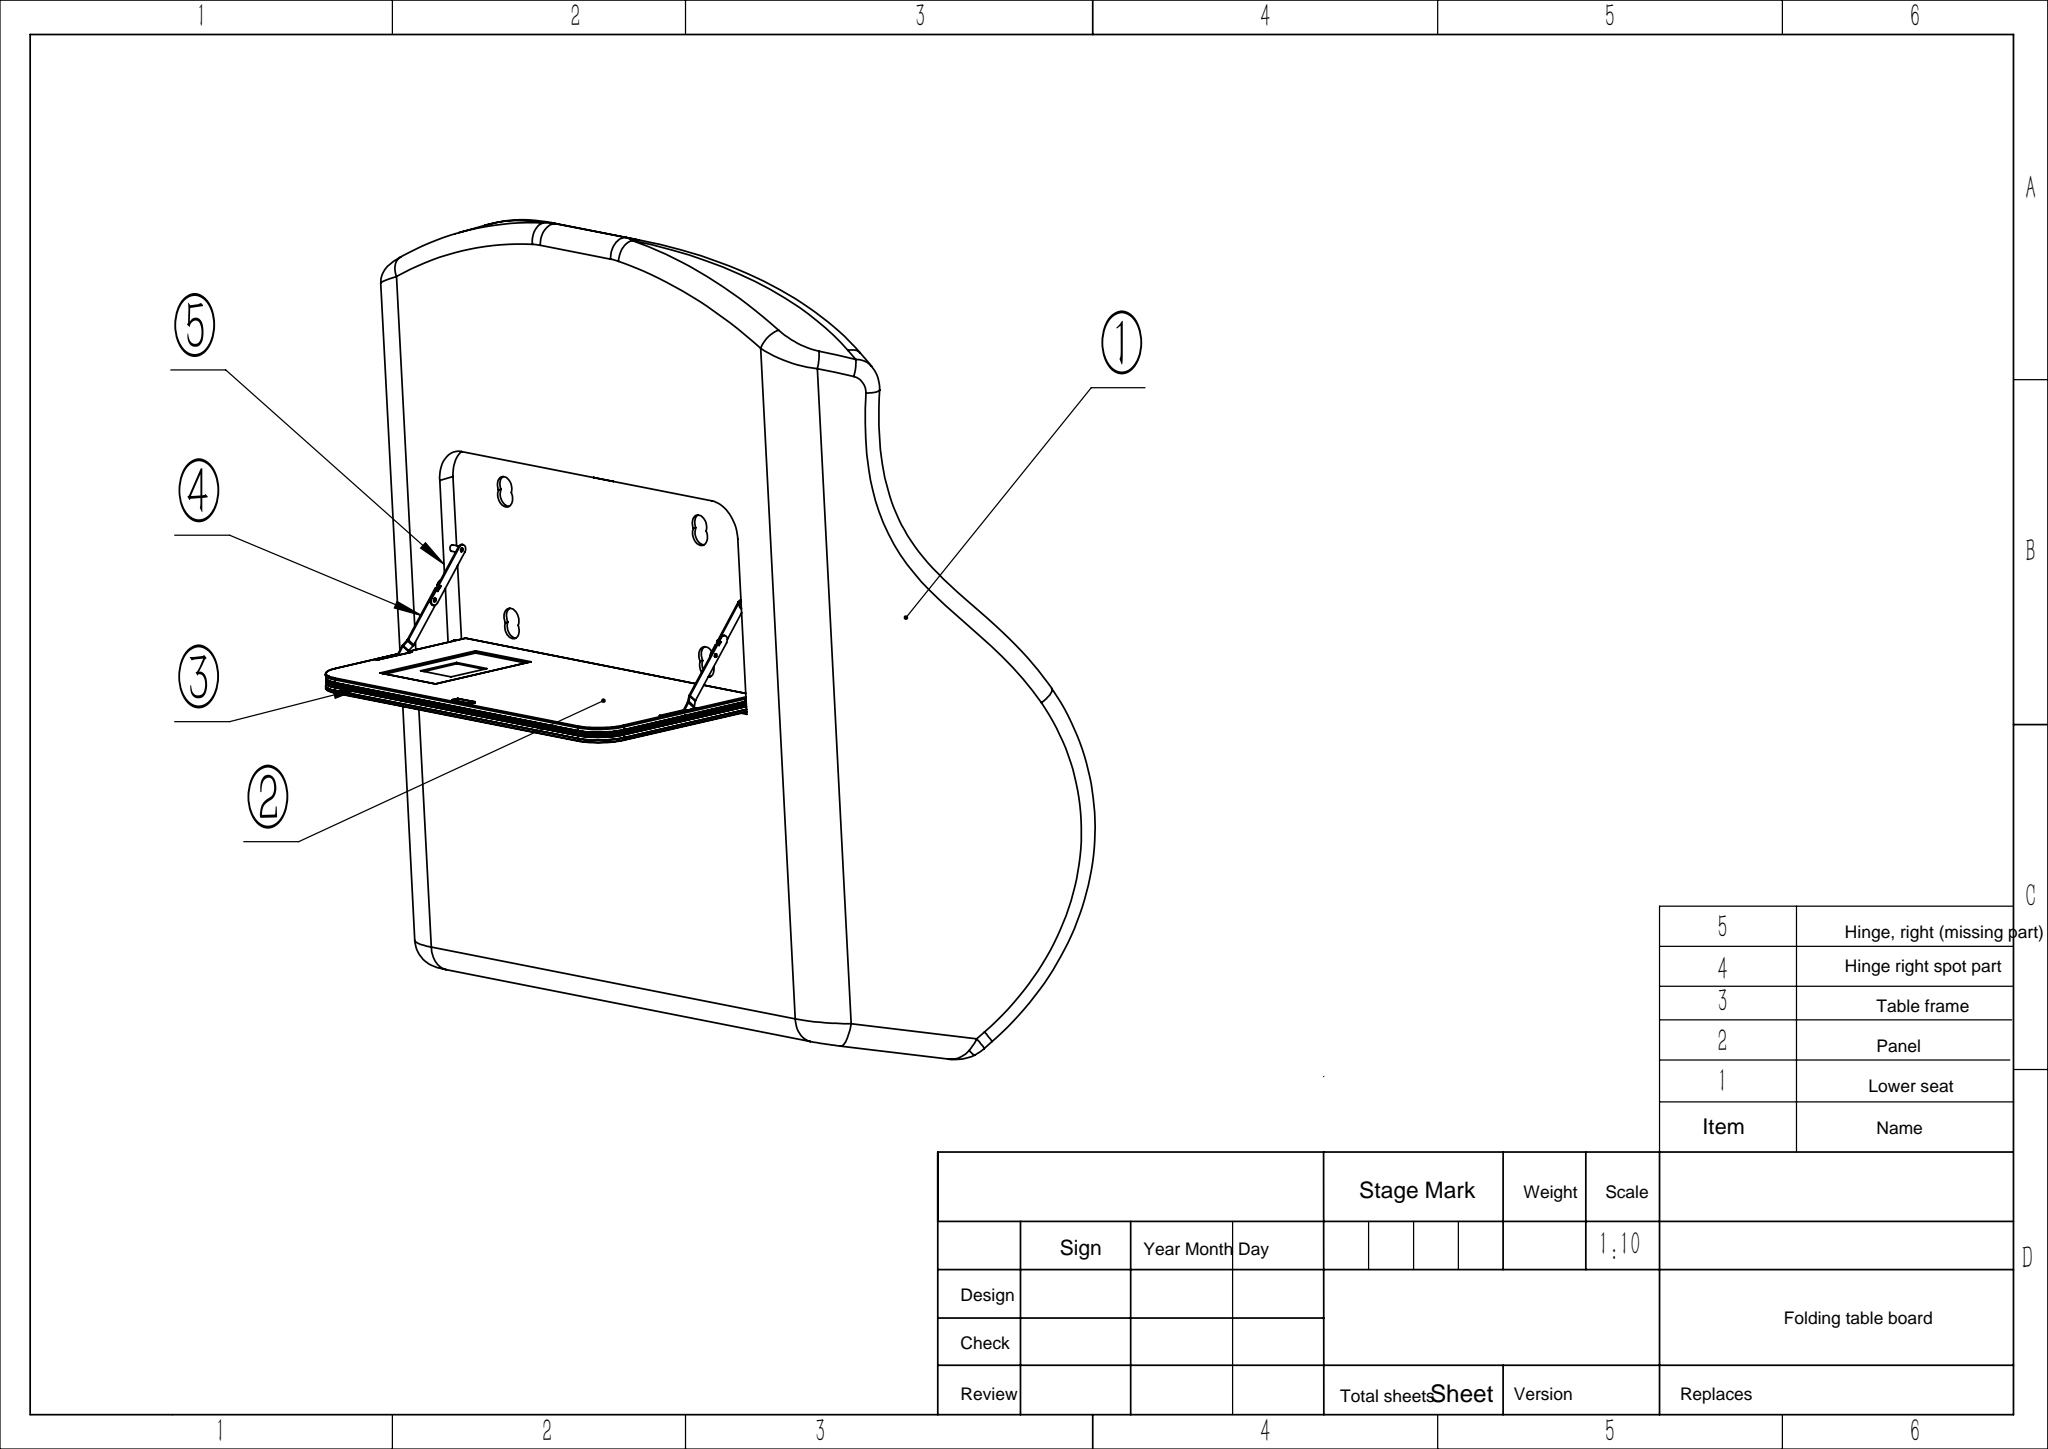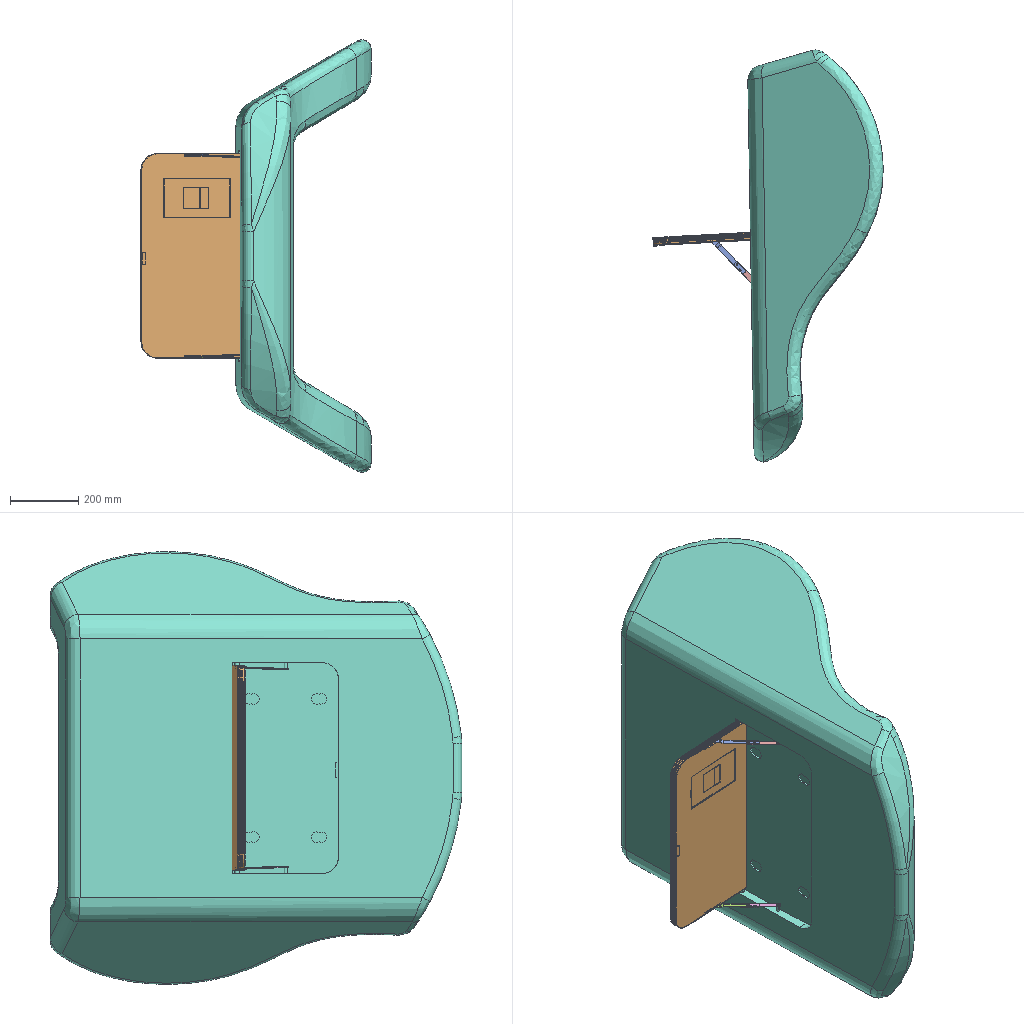Assembly | SolidWorks | 12 different items | 12 placed | box 674 x 1206 x 1267 mm
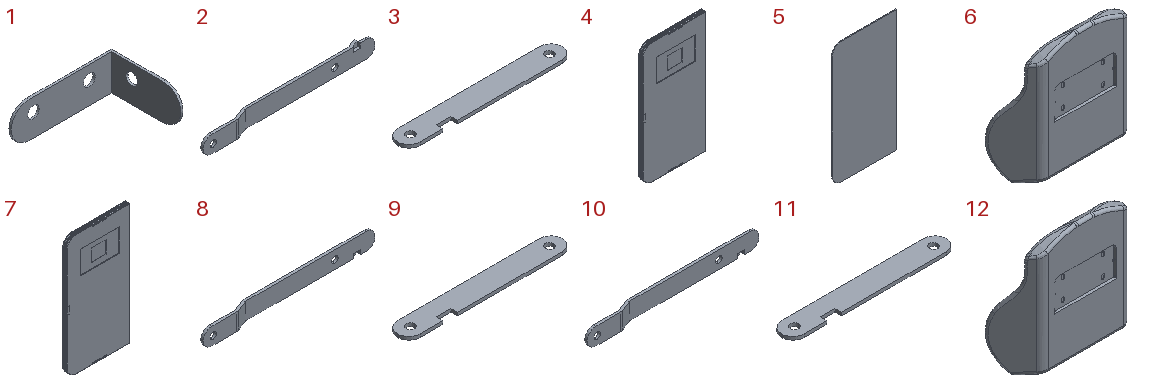Parts list (item | quantity | size | volume | features):
1 | x1 | 46 x 32 x 16 mm | 1113 mm3 | features MirrorStock 1
2 | x1 | 145 x 8.5 x 14 mm | 3916 mm3 | features MirrorStock 1
3 | x1 | 102 x 14 x 2 mm | 2615 mm3 | features MirrorStock 1
4 | x1 | 312 x 24.5 x 600 mm | 4043732 mm3 | features ICE 11, Fillet 4, MirrorPattern 1, Sweep 1
5 | x1 | 315.5 x 4 x 596 mm | 748519 mm3 | features Extrusion 1
6 | x1 | 1267 x 391.764 x 1203 mm | 196548846 mm3 | features ICE 13, MirrorPattern 6, Fillet 5, Extrusion 1, RefAxis 1, Scale 1
7 | x1 | 312 x 24.5 x 600 mm | 4043732 mm3 | features ICE 11, Fillet 4, MirrorPattern 1, Sweep 1
8 | x1 | 145 x 8.5 x 14 mm | 3916 mm3 | features ICE 3, Extrusion 1
9 | x1 | 102 x 14 x 2 mm | 2615 mm3 | features Extrusion 1
10 | x1 | 145 x 8.5 x 14 mm | 3916 mm3 | features ICE 3, Extrusion 1
11 | x1 | 102 x 14 x 2 mm | 2615 mm3 | features Extrusion 1
12 | x1 | 1267 x 391.764 x 1203 mm | 196548846 mm3 | features ICE 13, MirrorPattern 6, Fillet 5, Extrusion 1, RefAxis 1, Scale 1
Mates (type | each side: item.copy, entity, surface, feature):
Concentric | 11.1 face cylinder Extrude1 | 10.1 face cylinder Extrude2
Coincident | 11.1 face plane Extrude1 | 10.1 face plane Extrude1
LimitPlanarAngleDim | 10.1 face plane Extrude1 | 11.1 face plane Extrude1
DistanceDim | 11.1 face plane Extrude1 | 12.1 face plane Cut-Extrude1
Concentric | 11.1 face cylinder Extrude1 | 12.1 face cylinder Cut-Extrude3
Concentric | 3.1 face cylinder HingeRightMissing partMirror | 12.1 face cylinder Mirror1
Concentric | 12.1 face cylinder Mirror2 | 4.1 face cylinder Cut-Extrude3
Concentric | 12.1 face cylinder Cut-Extrude4 | 4.1 face cylinder Cut-Extrude3
DistanceDim | 4.1 face plane Sweep1 | 12.1 face plane Cut-Extrude1
Concentric | 10.1 face cylinder Extrude2 | 4.1 face cylinder Cut-Extrude6